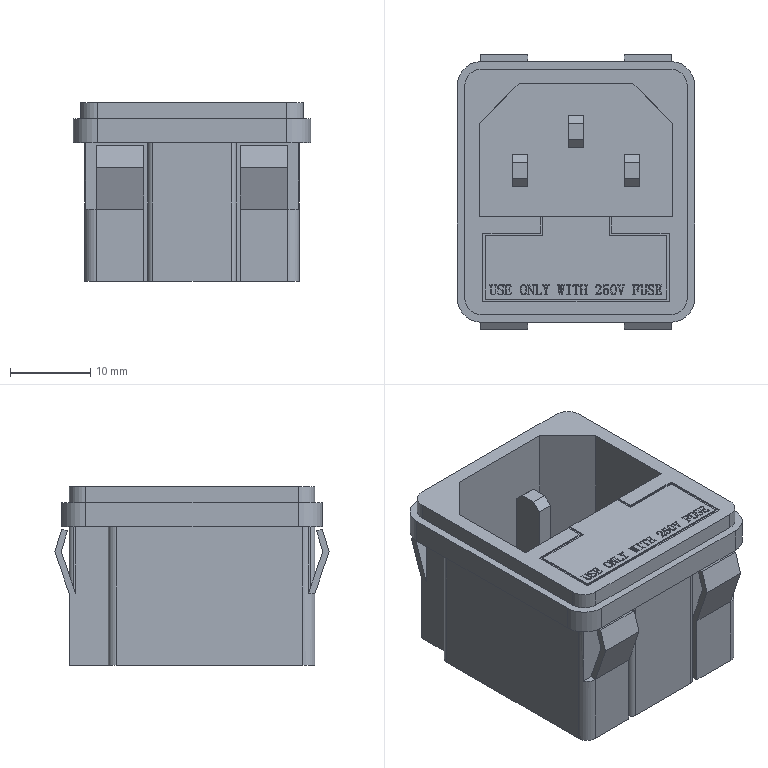Part | SolidWorks | features BaseBody 1 | 1 solid | 557 faces | box 29.6 x 34.2 x 22.3 mm | volume 11730 mm3 | plane 391 | spline 150 | cylinder 16 | commonest cylinder face diameters 1.2 x4 4.12 x4 6 x4 2 x2 3 x2